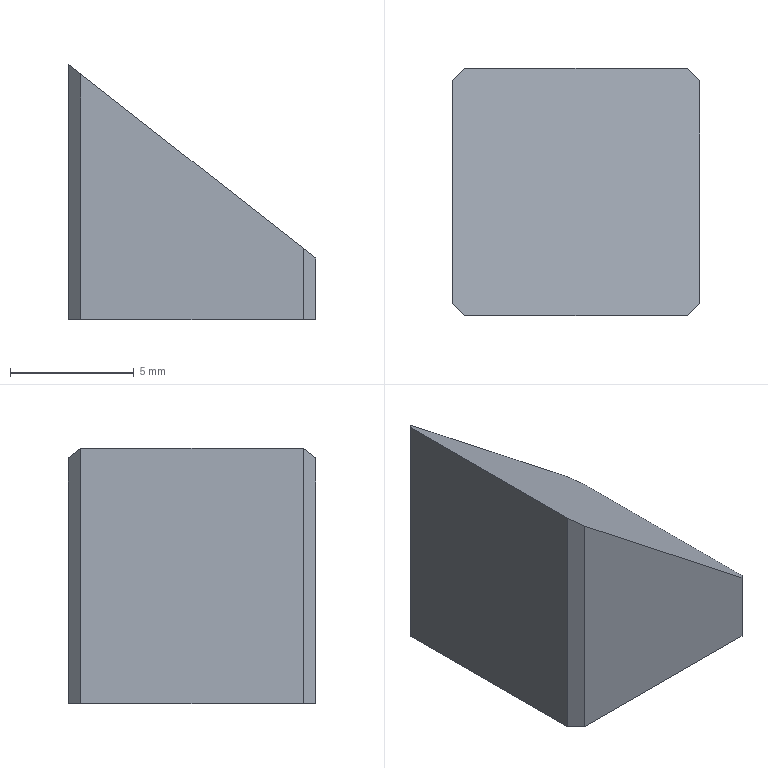Part | STEP file | GLP10-A.step.STEP.STEP-90.STEP | 1 solid | 10 faces | box 10 x 10 x 10.341 mm | volume 638.84 mm3 | plane 10
STEP:
#1=CARTESIAN_POINT('',(5.,-4.5,0.));
#2=VERTEX_POINT('',#1);
#3=CARTESIAN_POINT('',(5.,4.5,0.));
#4=VERTEX_POINT('',#3);
#5=CARTESIAN_POINT('',(5.,5.,0.));
#6=DIRECTION('',(0.,1.,0.));
#7=VECTOR('',#6,1000.);
#8=LINE('',#5,#7);
#9=EDGE_CURVE('',#2,#4,#8,.T.);
#10=ORIENTED_EDGE('',*,*,#9,.T.);
#11=CARTESIAN_POINT('',(5.,4.5,2.5));
#12=VERTEX_POINT('',#11);
#13=CARTESIAN_POINT('',(5.,4.5,20.));
#14=DIRECTION('',(0.,0.,1.));
#15=VECTOR('',#14,1000.);
#16=LINE('',#13,#15);
#17=EDGE_CURVE('',#4,#12,#16,.T.);
#18=ORIENTED_EDGE('',*,*,#17,.T.);
#19=CARTESIAN_POINT('',(5.,-4.5,2.5));
#20=VERTEX_POINT('',#19);
#21=CARTESIAN_POINT('',(5.,5.,2.5));
#22=DIRECTION('',(0.,-1.,0.));
#23=VECTOR('',#22,1000.);
#24=LINE('',#21,#23);
#25=EDGE_CURVE('',#12,#20,#24,.T.);
#26=ORIENTED_EDGE('',*,*,#25,.T.);
#27=CARTESIAN_POINT('',(5.,-4.5,20.));
#28=DIRECTION('',(0.,0.,-1.));
#29=VECTOR('',#28,1000.);
#30=LINE('',#27,#29);
#31=EDGE_CURVE('',#20,#2,#30,.T.);
#32=ORIENTED_EDGE('',*,*,#31,.T.);
#33=EDGE_LOOP('',(#10,#18,#26,#32));
#34=FACE_OUTER_BOUND('',#33,.T.);
#35=CARTESIAN_POINT('',(5.,5.,20.));
#36=DIRECTION('',(-1.,0.,0.));
#37=DIRECTION('',(0.,0.,1.));
#38=AXIS2_PLACEMENT_3D('',#35,#36,#37);
#39=PLANE('',#38);
#40=ADVANCED_FACE('',(#34),#39,.F.);
#41=CARTESIAN_POINT('',(4.5,5.,2.892));
#42=VERTEX_POINT('',#41);
#43=CARTESIAN_POINT('',(-4.5,5.,9.949));
#44=VERTEX_POINT('',#43);
#45=CARTESIAN_POINT('',(3.118,5.,3.976));
#46=DIRECTION('',(-0.7869,0.,0.617));
#47=VECTOR('',#46,1000.);
#48=LINE('',#45,#47);
#49=EDGE_CURVE('',#42,#44,#48,.T.);
#50=ORIENTED_EDGE('',*,*,#49,.F.);
#51=CARTESIAN_POINT('',(4.5,5.,0.));
#52=VERTEX_POINT('',#51);
#53=CARTESIAN_POINT('',(4.5,5.,20.));
#54=DIRECTION('',(0.,0.,-1.));
#55=VECTOR('',#54,1000.);
#56=LINE('',#53,#55);
#57=EDGE_CURVE('',#42,#52,#56,.T.);
#58=ORIENTED_EDGE('',*,*,#57,.T.);
#59=CARTESIAN_POINT('',(-4.5,5.,0.));
#60=VERTEX_POINT('',#59);
#61=CARTESIAN_POINT('',(-5.,5.,0.));
#62=DIRECTION('',(-1.,0.,0.));
#63=VECTOR('',#62,1000.);
#64=LINE('',#61,#63);
#65=EDGE_CURVE('',#52,#60,#64,.T.);
#66=ORIENTED_EDGE('',*,*,#65,.T.);
#67=CARTESIAN_POINT('',(-4.5,5.,20.));
#68=DIRECTION('',(0.,0.,1.));
#69=VECTOR('',#68,1000.);
#70=LINE('',#67,#69);
#71=EDGE_CURVE('',#60,#44,#70,.T.);
#72=ORIENTED_EDGE('',*,*,#71,.T.);
#73=EDGE_LOOP('',(#50,#58,#66,#72));
#74=FACE_OUTER_BOUND('',#73,.T.);
#75=CARTESIAN_POINT('',(-5.,5.,20.));
#76=DIRECTION('',(0.,-1.,0.));
#77=DIRECTION('',(0.,0.,-1.));
#78=AXIS2_PLACEMENT_3D('',#75,#76,#77);
#79=PLANE('',#78);
#80=ADVANCED_FACE('',(#74),#79,.F.);
#81=CARTESIAN_POINT('',(-5.,4.5,0.));
#82=VERTEX_POINT('',#81);
#83=CARTESIAN_POINT('',(-5.,-4.5,0.));
#84=VERTEX_POINT('',#83);
#85=CARTESIAN_POINT('',(-5.,5.,0.));
#86=DIRECTION('',(0.,-1.,0.));
#87=VECTOR('',#86,1000.);
#88=LINE('',#85,#87);
#89=EDGE_CURVE('',#82,#84,#88,.T.);
#90=ORIENTED_EDGE('',*,*,#89,.T.);
#91=CARTESIAN_POINT('',(-5.,-4.5,10.341));
#92=VERTEX_POINT('',#91);
#93=CARTESIAN_POINT('',(-5.,-4.5,20.));
#94=DIRECTION('',(0.,0.,1.));
#95=VECTOR('',#94,1000.);
#96=LINE('',#93,#95);
#97=EDGE_CURVE('',#84,#92,#96,.T.);
#98=ORIENTED_EDGE('',*,*,#97,.T.);
#99=CARTESIAN_POINT('',(-5.,4.5,10.341));
#100=VERTEX_POINT('',#99);
#101=CARTESIAN_POINT('',(-5.,5.,10.341));
#102=DIRECTION('',(0.,-1.,0.));
#103=VECTOR('',#102,1000.);
#104=LINE('',#101,#103);
#105=EDGE_CURVE('',#100,#92,#104,.T.);
#106=ORIENTED_EDGE('',*,*,#105,.F.);
#107=CARTESIAN_POINT('',(-5.,4.5,20.));
#108=DIRECTION('',(0.,0.,-1.));
#109=VECTOR('',#108,1000.);
#110=LINE('',#107,#109);
#111=EDGE_CURVE('',#100,#82,#110,.T.);
#112=ORIENTED_EDGE('',*,*,#111,.T.);
#113=EDGE_LOOP('',(#90,#98,#106,#112));
#114=FACE_OUTER_BOUND('',#113,.T.);
#115=CARTESIAN_POINT('',(-5.,5.,20.));
#116=DIRECTION('',(1.,0.,0.));
#117=DIRECTION('',(0.,1.,0.));
#118=AXIS2_PLACEMENT_3D('',#115,#116,#117);
#119=PLANE('',#118);
#120=ADVANCED_FACE('',(#114),#119,.F.);
#121=CARTESIAN_POINT('',(4.5,-5.,2.892));
#122=VERTEX_POINT('',#121);
#123=CARTESIAN_POINT('',(-4.5,-5.,9.949));
#124=VERTEX_POINT('',#123);
#125=CARTESIAN_POINT('',(3.118,-5.,3.976));
#126=DIRECTION('',(-0.7869,0.,0.617));
#127=VECTOR('',#126,1000.);
#128=LINE('',#125,#127);
#129=EDGE_CURVE('',#122,#124,#128,.T.);
#130=ORIENTED_EDGE('',*,*,#129,.T.);
#131=CARTESIAN_POINT('',(-4.5,-5.,0.));
#132=VERTEX_POINT('',#131);
#133=CARTESIAN_POINT('',(-4.5,-5.,20.));
#134=DIRECTION('',(0.,0.,-1.));
#135=VECTOR('',#134,1000.);
#136=LINE('',#133,#135);
#137=EDGE_CURVE('',#124,#132,#136,.T.);
#138=ORIENTED_EDGE('',*,*,#137,.T.);
#139=CARTESIAN_POINT('',(4.5,-5.,0.));
#140=VERTEX_POINT('',#139);
#141=CARTESIAN_POINT('',(-5.,-5.,0.));
#142=DIRECTION('',(1.,0.,0.));
#143=VECTOR('',#142,1000.);
#144=LINE('',#141,#143);
#145=EDGE_CURVE('',#132,#140,#144,.T.);
#146=ORIENTED_EDGE('',*,*,#145,.T.);
#147=CARTESIAN_POINT('',(4.5,-5.,20.));
#148=DIRECTION('',(0.,0.,1.));
#149=VECTOR('',#148,1000.);
#150=LINE('',#147,#149);
#151=EDGE_CURVE('',#140,#122,#150,.T.);
#152=ORIENTED_EDGE('',*,*,#151,.T.);
#153=EDGE_LOOP('',(#130,#138,#146,#152));
#154=FACE_OUTER_BOUND('',#153,.T.);
#155=CARTESIAN_POINT('',(-5.,-5.,20.));
#156=DIRECTION('',(0.,1.,0.));
#157=DIRECTION('',(1.,0.,0.));
#158=AXIS2_PLACEMENT_3D('',#155,#156,#157);
#159=PLANE('',#158);
#160=ADVANCED_FACE('',(#154),#159,.F.);
#161=ORIENTED_EDGE('',*,*,#65,.F.);
#162=CARTESIAN_POINT('',(4.5,5.,0.));
#163=DIRECTION('',(0.7071,-0.7071,0.));
#164=VECTOR('',#163,1000.);
#165=LINE('',#162,#164);
#166=EDGE_CURVE('',#52,#4,#165,.T.);
#167=ORIENTED_EDGE('',*,*,#166,.T.);
#168=ORIENTED_EDGE('',*,*,#9,.F.);
#169=CARTESIAN_POINT('',(5.,-4.5,0.));
#170=DIRECTION('',(-0.7071,-0.7071,0.));
#171=VECTOR('',#170,1000.);
#172=LINE('',#169,#171);
#173=EDGE_CURVE('',#2,#140,#172,.T.);
#174=ORIENTED_EDGE('',*,*,#173,.T.);
#175=ORIENTED_EDGE('',*,*,#145,.F.);
#176=CARTESIAN_POINT('',(-4.5,-5.,0.));
#177=DIRECTION('',(-0.7071,0.7071,0.));
#178=VECTOR('',#177,1000.);
#179=LINE('',#176,#178);
#180=EDGE_CURVE('',#132,#84,#179,.T.);
#181=ORIENTED_EDGE('',*,*,#180,.T.);
#182=ORIENTED_EDGE('',*,*,#89,.F.);
#183=CARTESIAN_POINT('',(-5.,4.5,0.));
#184=DIRECTION('',(0.7071,0.7071,0.));
#185=VECTOR('',#184,1000.);
#186=LINE('',#183,#185);
#187=EDGE_CURVE('',#82,#60,#186,.T.);
#188=ORIENTED_EDGE('',*,*,#187,.T.);
#189=EDGE_LOOP('',(#161,#167,#168,#174,#175,#181,#182,#188));
#190=FACE_OUTER_BOUND('',#189,.T.);
#191=CARTESIAN_POINT('',(0.,0.,0.));
#192=DIRECTION('',(0.,0.,1.));
#193=DIRECTION('',(1.,0.,0.));
#194=AXIS2_PLACEMENT_3D('',#191,#192,#193);
#195=PLANE('',#194);
#196=ADVANCED_FACE('',(#190),#195,.F.);
#197=ORIENTED_EDGE('',*,*,#25,.F.);
#198=CARTESIAN_POINT('',(3.646,5.854,3.561));
#199=DIRECTION('',(-0.6184,0.6184,0.4849));
#200=VECTOR('',#199,1000.);
#201=LINE('',#198,#200);
#202=EDGE_CURVE('',#12,#42,#201,.T.);
#203=ORIENTED_EDGE('',*,*,#202,.T.);
#204=ORIENTED_EDGE('',*,*,#49,.T.);
#205=CARTESIAN_POINT('',(0.2043,9.704,6.26));
#206=DIRECTION('',(-0.6184,-0.6184,0.4849));
#207=VECTOR('',#206,1000.);
#208=LINE('',#205,#207);
#209=EDGE_CURVE('',#44,#100,#208,.T.);
#210=ORIENTED_EDGE('',*,*,#209,.T.);
#211=ORIENTED_EDGE('',*,*,#105,.T.);
#212=CARTESIAN_POINT('',(-3.62,-5.88,9.259));
#213=DIRECTION('',(0.6184,-0.6184,-0.4849));
#214=VECTOR('',#213,1000.);
#215=LINE('',#212,#214);
#216=EDGE_CURVE('',#92,#124,#215,.T.);
#217=ORIENTED_EDGE('',*,*,#216,.T.);
#218=ORIENTED_EDGE('',*,*,#129,.F.);
#219=CARTESIAN_POINT('',(7.471,-2.029,0.5628));
#220=DIRECTION('',(0.6184,0.6184,-0.4849));
#221=VECTOR('',#220,1000.);
#222=LINE('',#219,#221);
#223=EDGE_CURVE('',#122,#20,#222,.T.);
#224=ORIENTED_EDGE('',*,*,#223,.T.);
#225=EDGE_LOOP('',(#197,#203,#204,#210,#211,#217,#218,#224));
#226=FACE_OUTER_BOUND('',#225,.T.);
#227=CARTESIAN_POINT('',(3.118,5.,3.976));
#228=DIRECTION('',(0.617,0.,0.7869));
#229=DIRECTION('',(0.,-1.,0.));
#230=AXIS2_PLACEMENT_3D('',#227,#228,#229);
#231=PLANE('',#230);
#232=ADVANCED_FACE('',(#226),#231,.T.);
#233=ORIENTED_EDGE('',*,*,#202,.F.);
#234=ORIENTED_EDGE('',*,*,#17,.F.);
#235=ORIENTED_EDGE('',*,*,#166,.F.);
#236=ORIENTED_EDGE('',*,*,#57,.F.);
#237=EDGE_LOOP('',(#233,#234,#235,#236));
#238=FACE_OUTER_BOUND('',#237,.T.);
#239=CARTESIAN_POINT('',(4.5,5.,20.));
#240=DIRECTION('',(-0.7071,-0.7071,0.));
#241=DIRECTION('',(-0.7071,0.7071,0.));
#242=AXIS2_PLACEMENT_3D('',#239,#240,#241);
#243=PLANE('',#242);
#244=ADVANCED_FACE('',(#238),#243,.F.);
#245=ORIENTED_EDGE('',*,*,#216,.F.);
#246=ORIENTED_EDGE('',*,*,#97,.F.);
#247=ORIENTED_EDGE('',*,*,#180,.F.);
#248=ORIENTED_EDGE('',*,*,#137,.F.);
#249=EDGE_LOOP('',(#245,#246,#247,#248));
#250=FACE_OUTER_BOUND('',#249,.T.);
#251=CARTESIAN_POINT('',(-4.5,-5.,20.));
#252=DIRECTION('',(0.7071,0.7071,0.));
#253=DIRECTION('',(0.,0.,-1.));
#254=AXIS2_PLACEMENT_3D('',#251,#252,#253);
#255=PLANE('',#254);
#256=ADVANCED_FACE('',(#250),#255,.F.);
#257=ORIENTED_EDGE('',*,*,#223,.F.);
#258=ORIENTED_EDGE('',*,*,#151,.F.);
#259=ORIENTED_EDGE('',*,*,#173,.F.);
#260=ORIENTED_EDGE('',*,*,#31,.F.);
#261=EDGE_LOOP('',(#257,#258,#259,#260));
#262=FACE_OUTER_BOUND('',#261,.T.);
#263=CARTESIAN_POINT('',(5.,-4.5,20.));
#264=DIRECTION('',(-0.7071,0.7071,0.));
#265=DIRECTION('',(0.,0.,1.));
#266=AXIS2_PLACEMENT_3D('',#263,#264,#265);
#267=PLANE('',#266);
#268=ADVANCED_FACE('',(#262),#267,.F.);
#269=ORIENTED_EDGE('',*,*,#209,.F.);
#270=ORIENTED_EDGE('',*,*,#71,.F.);
#271=ORIENTED_EDGE('',*,*,#187,.F.);
#272=ORIENTED_EDGE('',*,*,#111,.F.);
#273=EDGE_LOOP('',(#269,#270,#271,#272));
#274=FACE_OUTER_BOUND('',#273,.T.);
#275=CARTESIAN_POINT('',(-5.,4.5,20.));
#276=DIRECTION('',(0.7071,-0.7071,0.));
#277=DIRECTION('',(0.,0.,-1.));
#278=AXIS2_PLACEMENT_3D('',#275,#276,#277);
#279=PLANE('',#278);
#280=ADVANCED_FACE('',(#274),#279,.F.);
#281=CLOSED_SHELL('',(#40,#80,#120,#160,#196,#232,#244,#256,#268,#280));
#282=MANIFOLD_SOLID_BREP('',#281);
#283=CARTESIAN_POINT('',(0.,0.,0.));
#284=DIRECTION('',(0.,0.,1.));
#285=DIRECTION('',(1.,0.,0.));
#286=AXIS2_PLACEMENT_3D('',#283,#284,#285);
#287=(LENGTH_UNIT()NAMED_UNIT(*)SI_UNIT(.MILLI.,.METRE.));
#288=UNCERTAINTY_MEASURE_WITH_UNIT(LENGTH_MEASURE(0.00001),#287,'','');
#289=(NAMED_UNIT(*)PLANE_ANGLE_UNIT()SI_UNIT($,.RADIAN.));
#290=(NAMED_UNIT(*)SI_UNIT($,.STERADIAN.)SOLID_ANGLE_UNIT());
#291=(GEOMETRIC_REPRESENTATION_CONTEXT(3)GLOBAL_UNCERTAINTY_ASSIGNED_CONTEXT((#288))GLOBAL_UNIT_ASSIGNED_CONTEXT((#287,#289,#290))REPRESENTATION_CONTEXT('',''));
#292=ADVANCED_BREP_SHAPE_REPRESENTATION('',(#282,#286),#291);